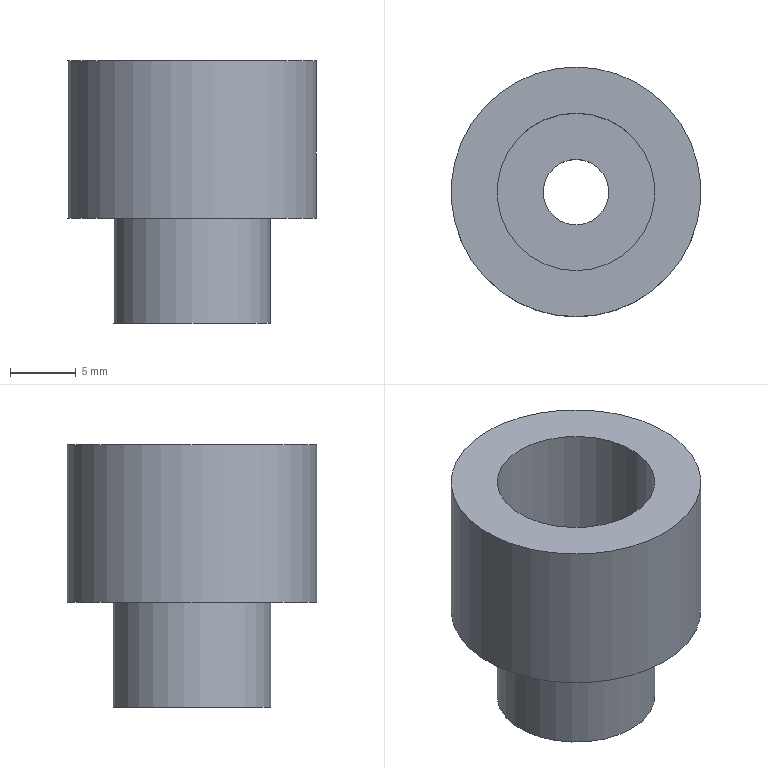Part | STEP file | 1-16.6 | 1 solid | 8 faces | box 19 x 19 x 20 mm | volume 2980 mm3 | cylinder 4 | plane 4 | commonest cylinder face diameters 12 x2 5 x1 19 x1
STEP:
#1=CARTESIAN_POINT('',(0.,0.,0.));
#2=DIRECTION('',(0.,0.,1.));
#3=DIRECTION('',(1.,0.,0.));
#4=AXIS2_PLACEMENT_3D('',#1,#2,#3);
#5=CARTESIAN_POINT('',(0.,9.5,0.));
#6=VERTEX_POINT('',#5);
#7=CARTESIAN_POINT('',(0.,0.,0.));
#8=DIRECTION('',(0.,0.,1.));
#9=DIRECTION('',(0.,1.,0.));
#10=AXIS2_PLACEMENT_3D('',#7,#8,#9);
#11=CIRCLE('',#10,9.5);
#12=CARTESIAN_POINT('',(0.,0.,0.));
#13=DIRECTION('',(0.,0.,1.));
#14=DIRECTION('',(0.,1.,0.));
#15=AXIS2_PLACEMENT_3D('',#12,#13,#14);
#16=CYLINDRICAL_SURFACE('',#15,9.5);
#17=CARTESIAN_POINT('',(0.,0.));
#18=DIRECTION('',(1.,0.));
#19=VECTOR('',#18,1.);
#20=LINE('',#17,#19);
#21=(GEOMETRIC_REPRESENTATION_CONTEXT(2)PARAMETRIC_REPRESENTATION_CONTEXT()REPRESENTATION_CONTEXT('',''));
#22=DEFINITIONAL_REPRESENTATION('',(#20),#21);
#23=PCURVE('',#16,#22);
#24=CARTESIAN_POINT('',(0.,-2.546,0.));
#25=DIRECTION('',(0.,0.,1.));
#26=DIRECTION('',(1.,0.,0.));
#27=AXIS2_PLACEMENT_3D('',#24,#25,#26);
#28=PLANE('',#27);
#29=CARTESIAN_POINT('',(0.,2.546));
#30=DIRECTION('',(0.,1.));
#31=AXIS2_PLACEMENT_2D('',#29,#30);
#32=CIRCLE('',#31,9.5);
#33=(GEOMETRIC_REPRESENTATION_CONTEXT(2)PARAMETRIC_REPRESENTATION_CONTEXT()REPRESENTATION_CONTEXT('',''));
#34=DEFINITIONAL_REPRESENTATION('',(#32),#33);
#35=PCURVE('',#28,#34);
#36=SURFACE_CURVE('',#11,(#23,#35),.PCURVE_S1.);
#37=EDGE_CURVE('',#6,#6,#36,.T.);
#38=ORIENTED_EDGE('',*,*,#37,.T.);
#39=CARTESIAN_POINT('',(0.,9.5,12.));
#40=VERTEX_POINT('',#39);
#41=CARTESIAN_POINT('',(0.,9.5,0.));
#42=DIRECTION('',(0.,0.,1.));
#43=VECTOR('',#42,1.);
#44=LINE('',#41,#43);
#45=CARTESIAN_POINT('',(6.283,0.));
#46=DIRECTION('',(0.,1.));
#47=VECTOR('',#46,1.);
#48=LINE('',#45,#47);
#49=(GEOMETRIC_REPRESENTATION_CONTEXT(2)PARAMETRIC_REPRESENTATION_CONTEXT()REPRESENTATION_CONTEXT('',''));
#50=DEFINITIONAL_REPRESENTATION('',(#48),#49);
#51=PCURVE('',#16,#50);
#52=CARTESIAN_POINT('',(0.,0.));
#53=DIRECTION('',(0.,1.));
#54=VECTOR('',#53,1.);
#55=LINE('',#52,#54);
#56=(GEOMETRIC_REPRESENTATION_CONTEXT(2)PARAMETRIC_REPRESENTATION_CONTEXT()REPRESENTATION_CONTEXT('',''));
#57=DEFINITIONAL_REPRESENTATION('',(#55),#56);
#58=PCURVE('',#16,#57);
#59=SEAM_CURVE('',#44,(#51,#58),.PCURVE_S1.);
#60=EDGE_CURVE('',#6,#40,#59,.T.);
#61=ORIENTED_EDGE('',*,*,#60,.T.);
#62=CARTESIAN_POINT('',(0.,0.,12.));
#63=DIRECTION('',(0.,0.,1.));
#64=DIRECTION('',(0.,1.,0.));
#65=AXIS2_PLACEMENT_3D('',#62,#63,#64);
#66=CIRCLE('',#65,9.5);
#67=CARTESIAN_POINT('',(0.,12.));
#68=DIRECTION('',(1.,0.));
#69=VECTOR('',#68,1.);
#70=LINE('',#67,#69);
#71=(GEOMETRIC_REPRESENTATION_CONTEXT(2)PARAMETRIC_REPRESENTATION_CONTEXT()REPRESENTATION_CONTEXT('',''));
#72=DEFINITIONAL_REPRESENTATION('',(#70),#71);
#73=PCURVE('',#16,#72);
#74=CARTESIAN_POINT('',(0.,-2.546,12.));
#75=DIRECTION('',(0.,0.,1.));
#76=DIRECTION('',(1.,0.,0.));
#77=AXIS2_PLACEMENT_3D('',#74,#75,#76);
#78=PLANE('',#77);
#79=CARTESIAN_POINT('',(0.,2.546));
#80=DIRECTION('',(0.,1.));
#81=AXIS2_PLACEMENT_2D('',#79,#80);
#82=CIRCLE('',#81,9.5);
#83=(GEOMETRIC_REPRESENTATION_CONTEXT(2)PARAMETRIC_REPRESENTATION_CONTEXT()REPRESENTATION_CONTEXT('',''));
#84=DEFINITIONAL_REPRESENTATION('',(#82),#83);
#85=PCURVE('',#78,#84);
#86=SURFACE_CURVE('',#66,(#73,#85),.PCURVE_S1.);
#87=EDGE_CURVE('',#40,#40,#86,.T.);
#88=ORIENTED_EDGE('',*,*,#87,.F.);
#89=ORIENTED_EDGE('',*,*,#60,.F.);
#90=EDGE_LOOP('',(#38,#61,#88,#89));
#91=FACE_BOUND('',#90,.T.);
#92=ADVANCED_FACE('',(#91),#16,.T.);
#93=ORIENTED_EDGE('',*,*,#37,.T.);
#94=EDGE_LOOP('',(#93));
#95=FACE_BOUND('',#94,.F.);
#96=CARTESIAN_POINT('',(0.,6.,0.));
#97=VERTEX_POINT('',#96);
#98=CARTESIAN_POINT('',(0.,0.,0.));
#99=DIRECTION('',(0.,0.,1.));
#100=DIRECTION('',(0.,1.,0.));
#101=AXIS2_PLACEMENT_3D('',#98,#99,#100);
#102=CIRCLE('',#101,6.);
#103=CARTESIAN_POINT('',(0.,2.546));
#104=DIRECTION('',(0.,1.));
#105=AXIS2_PLACEMENT_2D('',#103,#104);
#106=CIRCLE('',#105,6.);
#107=(GEOMETRIC_REPRESENTATION_CONTEXT(2)PARAMETRIC_REPRESENTATION_CONTEXT()REPRESENTATION_CONTEXT('',''));
#108=DEFINITIONAL_REPRESENTATION('',(#106),#107);
#109=PCURVE('',#28,#108);
#110=CARTESIAN_POINT('',(0.,0.,0.));
#111=DIRECTION('',(0.,0.,-1.));
#112=DIRECTION('',(0.,1.,0.));
#113=AXIS2_PLACEMENT_3D('',#110,#111,#112);
#114=CYLINDRICAL_SURFACE('',#113,6.);
#115=CARTESIAN_POINT('',(6.283,0.));
#116=DIRECTION('',(-1.,0.));
#117=VECTOR('',#116,1.);
#118=LINE('',#115,#117);
#119=(GEOMETRIC_REPRESENTATION_CONTEXT(2)PARAMETRIC_REPRESENTATION_CONTEXT()REPRESENTATION_CONTEXT('',''));
#120=DEFINITIONAL_REPRESENTATION('',(#118),#119);
#121=PCURVE('',#114,#120);
#122=SURFACE_CURVE('',#102,(#109,#121),.PCURVE_S1.);
#123=EDGE_CURVE('',#97,#97,#122,.T.);
#124=ORIENTED_EDGE('',*,*,#123,.F.);
#125=EDGE_LOOP('',(#124));
#126=FACE_BOUND('',#125,.F.);
#127=ADVANCED_FACE('',(#95,#126),#28,.F.);
#128=CARTESIAN_POINT('',(0.,6.,-8.));
#129=VERTEX_POINT('',#128);
#130=CARTESIAN_POINT('',(0.,6.,0.));
#131=DIRECTION('',(0.,0.,-1.));
#132=VECTOR('',#131,1.);
#133=LINE('',#130,#132);
#134=CARTESIAN_POINT('',(6.283,0.));
#135=DIRECTION('',(0.,1.));
#136=VECTOR('',#135,1.);
#137=LINE('',#134,#136);
#138=(GEOMETRIC_REPRESENTATION_CONTEXT(2)PARAMETRIC_REPRESENTATION_CONTEXT()REPRESENTATION_CONTEXT('',''));
#139=DEFINITIONAL_REPRESENTATION('',(#137),#138);
#140=PCURVE('',#114,#139);
#141=CARTESIAN_POINT('',(0.,0.));
#142=DIRECTION('',(0.,1.));
#143=VECTOR('',#142,1.);
#144=LINE('',#141,#143);
#145=(GEOMETRIC_REPRESENTATION_CONTEXT(2)PARAMETRIC_REPRESENTATION_CONTEXT()REPRESENTATION_CONTEXT('',''));
#146=DEFINITIONAL_REPRESENTATION('',(#144),#145);
#147=PCURVE('',#114,#146);
#148=SEAM_CURVE('',#133,(#140,#147),.PCURVE_S1.);
#149=EDGE_CURVE('',#97,#129,#148,.T.);
#150=ORIENTED_EDGE('',*,*,#149,.T.);
#151=CARTESIAN_POINT('',(0.,0.,-8.));
#152=DIRECTION('',(0.,0.,1.));
#153=DIRECTION('',(0.,1.,0.));
#154=AXIS2_PLACEMENT_3D('',#151,#152,#153);
#155=CIRCLE('',#154,6.);
#156=CARTESIAN_POINT('',(6.283,8.));
#157=DIRECTION('',(-1.,0.));
#158=VECTOR('',#157,1.);
#159=LINE('',#156,#158);
#160=(GEOMETRIC_REPRESENTATION_CONTEXT(2)PARAMETRIC_REPRESENTATION_CONTEXT()REPRESENTATION_CONTEXT('',''));
#161=DEFINITIONAL_REPRESENTATION('',(#159),#160);
#162=PCURVE('',#114,#161);
#163=CARTESIAN_POINT('',(0.,-1.608,-8.));
#164=DIRECTION('',(0.,0.,1.));
#165=DIRECTION('',(1.,0.,0.));
#166=AXIS2_PLACEMENT_3D('',#163,#164,#165);
#167=PLANE('',#166);
#168=CARTESIAN_POINT('',(0.,1.608));
#169=DIRECTION('',(0.,1.));
#170=AXIS2_PLACEMENT_2D('',#168,#169);
#171=CIRCLE('',#170,6.);
#172=(GEOMETRIC_REPRESENTATION_CONTEXT(2)PARAMETRIC_REPRESENTATION_CONTEXT()REPRESENTATION_CONTEXT('',''));
#173=DEFINITIONAL_REPRESENTATION('',(#171),#172);
#174=PCURVE('',#167,#173);
#175=SURFACE_CURVE('',#155,(#162,#174),.PCURVE_S1.);
#176=EDGE_CURVE('',#129,#129,#175,.T.);
#177=ORIENTED_EDGE('',*,*,#176,.T.);
#178=ORIENTED_EDGE('',*,*,#149,.F.);
#179=ORIENTED_EDGE('',*,*,#123,.F.);
#180=EDGE_LOOP('',(#150,#177,#178,#179));
#181=FACE_BOUND('',#180,.T.);
#182=ADVANCED_FACE('',(#181),#114,.T.);
#183=ORIENTED_EDGE('',*,*,#87,.T.);
#184=EDGE_LOOP('',(#183));
#185=FACE_BOUND('',#184,.T.);
#186=CARTESIAN_POINT('',(0.,6.,12.));
#187=VERTEX_POINT('',#186);
#188=CARTESIAN_POINT('',(0.,0.,12.));
#189=DIRECTION('',(0.,0.,1.));
#190=DIRECTION('',(0.,1.,0.));
#191=AXIS2_PLACEMENT_3D('',#188,#189,#190);
#192=CIRCLE('',#191,6.);
#193=CARTESIAN_POINT('',(0.,2.546));
#194=DIRECTION('',(0.,1.));
#195=AXIS2_PLACEMENT_2D('',#193,#194);
#196=CIRCLE('',#195,6.);
#197=(GEOMETRIC_REPRESENTATION_CONTEXT(2)PARAMETRIC_REPRESENTATION_CONTEXT()REPRESENTATION_CONTEXT('',''));
#198=DEFINITIONAL_REPRESENTATION('',(#196),#197);
#199=PCURVE('',#78,#198);
#200=CARTESIAN_POINT('',(0.,0.,12.));
#201=DIRECTION('',(0.,0.,-1.));
#202=DIRECTION('',(0.,1.,0.));
#203=AXIS2_PLACEMENT_3D('',#200,#201,#202);
#204=CYLINDRICAL_SURFACE('',#203,6.);
#205=CARTESIAN_POINT('',(6.283,0.));
#206=DIRECTION('',(-1.,0.));
#207=VECTOR('',#206,1.);
#208=LINE('',#205,#207);
#209=(GEOMETRIC_REPRESENTATION_CONTEXT(2)PARAMETRIC_REPRESENTATION_CONTEXT()REPRESENTATION_CONTEXT('',''));
#210=DEFINITIONAL_REPRESENTATION('',(#208),#209);
#211=PCURVE('',#204,#210);
#212=SURFACE_CURVE('',#192,(#199,#211),.PCURVE_S1.);
#213=EDGE_CURVE('',#187,#187,#212,.T.);
#214=ORIENTED_EDGE('',*,*,#213,.F.);
#215=EDGE_LOOP('',(#214));
#216=FACE_BOUND('',#215,.T.);
#217=ADVANCED_FACE('',(#185,#216),#78,.T.);
#218=CARTESIAN_POINT('',(0.,6.,2.));
#219=VERTEX_POINT('',#218);
#220=CARTESIAN_POINT('',(0.,6.,12.));
#221=DIRECTION('',(0.,0.,-1.));
#222=VECTOR('',#221,1.);
#223=LINE('',#220,#222);
#224=CARTESIAN_POINT('',(6.283,0.));
#225=DIRECTION('',(0.,1.));
#226=VECTOR('',#225,1.);
#227=LINE('',#224,#226);
#228=(GEOMETRIC_REPRESENTATION_CONTEXT(2)PARAMETRIC_REPRESENTATION_CONTEXT()REPRESENTATION_CONTEXT('',''));
#229=DEFINITIONAL_REPRESENTATION('',(#227),#228);
#230=PCURVE('',#204,#229);
#231=CARTESIAN_POINT('',(0.,0.));
#232=DIRECTION('',(0.,1.));
#233=VECTOR('',#232,1.);
#234=LINE('',#231,#233);
#235=(GEOMETRIC_REPRESENTATION_CONTEXT(2)PARAMETRIC_REPRESENTATION_CONTEXT()REPRESENTATION_CONTEXT('',''));
#236=DEFINITIONAL_REPRESENTATION('',(#234),#235);
#237=PCURVE('',#204,#236);
#238=SEAM_CURVE('',#223,(#230,#237),.PCURVE_S1.);
#239=EDGE_CURVE('',#187,#219,#238,.T.);
#240=ORIENTED_EDGE('',*,*,#239,.T.);
#241=CARTESIAN_POINT('',(0.,0.,2.));
#242=DIRECTION('',(0.,0.,1.));
#243=DIRECTION('',(0.,1.,0.));
#244=AXIS2_PLACEMENT_3D('',#241,#242,#243);
#245=CIRCLE('',#244,6.);
#246=CARTESIAN_POINT('',(6.283,10.));
#247=DIRECTION('',(-1.,0.));
#248=VECTOR('',#247,1.);
#249=LINE('',#246,#248);
#250=(GEOMETRIC_REPRESENTATION_CONTEXT(2)PARAMETRIC_REPRESENTATION_CONTEXT()REPRESENTATION_CONTEXT('',''));
#251=DEFINITIONAL_REPRESENTATION('',(#249),#250);
#252=PCURVE('',#204,#251);
#253=CARTESIAN_POINT('',(0.,-1.608,2.));
#254=DIRECTION('',(0.,0.,1.));
#255=DIRECTION('',(1.,0.,0.));
#256=AXIS2_PLACEMENT_3D('',#253,#254,#255);
#257=PLANE('',#256);
#258=CARTESIAN_POINT('',(0.,1.608));
#259=DIRECTION('',(0.,1.));
#260=AXIS2_PLACEMENT_2D('',#258,#259);
#261=CIRCLE('',#260,6.);
#262=(GEOMETRIC_REPRESENTATION_CONTEXT(2)PARAMETRIC_REPRESENTATION_CONTEXT()REPRESENTATION_CONTEXT('',''));
#263=DEFINITIONAL_REPRESENTATION('',(#261),#262);
#264=PCURVE('',#257,#263);
#265=SURFACE_CURVE('',#245,(#252,#264),.PCURVE_S1.);
#266=EDGE_CURVE('',#219,#219,#265,.T.);
#267=ORIENTED_EDGE('',*,*,#266,.T.);
#268=ORIENTED_EDGE('',*,*,#239,.F.);
#269=ORIENTED_EDGE('',*,*,#213,.F.);
#270=EDGE_LOOP('',(#240,#267,#268,#269));
#271=FACE_BOUND('',#270,.F.);
#272=ADVANCED_FACE('',(#271),#204,.F.);
#273=ORIENTED_EDGE('',*,*,#176,.T.);
#274=EDGE_LOOP('',(#273));
#275=FACE_BOUND('',#274,.F.);
#276=CARTESIAN_POINT('',(0.,2.5,-8.));
#277=VERTEX_POINT('',#276);
#278=CARTESIAN_POINT('',(0.,0.,-8.));
#279=DIRECTION('',(0.,0.,1.));
#280=DIRECTION('',(0.,1.,0.));
#281=AXIS2_PLACEMENT_3D('',#278,#279,#280);
#282=CIRCLE('',#281,2.5);
#283=CARTESIAN_POINT('',(0.,1.608));
#284=DIRECTION('',(0.,1.));
#285=AXIS2_PLACEMENT_2D('',#283,#284);
#286=CIRCLE('',#285,2.5);
#287=(GEOMETRIC_REPRESENTATION_CONTEXT(2)PARAMETRIC_REPRESENTATION_CONTEXT()REPRESENTATION_CONTEXT('',''));
#288=DEFINITIONAL_REPRESENTATION('',(#286),#287);
#289=PCURVE('',#167,#288);
#290=CARTESIAN_POINT('',(0.,0.,12.));
#291=DIRECTION('',(0.,0.,-1.));
#292=DIRECTION('',(0.,1.,0.));
#293=AXIS2_PLACEMENT_3D('',#290,#291,#292);
#294=CYLINDRICAL_SURFACE('',#293,2.5);
#295=CARTESIAN_POINT('',(6.283,20.));
#296=DIRECTION('',(-1.,0.));
#297=VECTOR('',#296,1.);
#298=LINE('',#295,#297);
#299=(GEOMETRIC_REPRESENTATION_CONTEXT(2)PARAMETRIC_REPRESENTATION_CONTEXT()REPRESENTATION_CONTEXT('',''));
#300=DEFINITIONAL_REPRESENTATION('',(#298),#299);
#301=PCURVE('',#294,#300);
#302=SURFACE_CURVE('',#282,(#289,#301),.PCURVE_S1.);
#303=EDGE_CURVE('',#277,#277,#302,.T.);
#304=ORIENTED_EDGE('',*,*,#303,.F.);
#305=EDGE_LOOP('',(#304));
#306=FACE_BOUND('',#305,.F.);
#307=ADVANCED_FACE('',(#275,#306),#167,.F.);
#308=ORIENTED_EDGE('',*,*,#266,.T.);
#309=EDGE_LOOP('',(#308));
#310=FACE_BOUND('',#309,.T.);
#311=CARTESIAN_POINT('',(0.,2.5,2.));
#312=VERTEX_POINT('',#311);
#313=CARTESIAN_POINT('',(0.,0.,2.));
#314=DIRECTION('',(0.,0.,1.));
#315=DIRECTION('',(0.,1.,0.));
#316=AXIS2_PLACEMENT_3D('',#313,#314,#315);
#317=CIRCLE('',#316,2.5);
#318=CARTESIAN_POINT('',(0.,1.608));
#319=DIRECTION('',(0.,1.));
#320=AXIS2_PLACEMENT_2D('',#318,#319);
#321=CIRCLE('',#320,2.5);
#322=(GEOMETRIC_REPRESENTATION_CONTEXT(2)PARAMETRIC_REPRESENTATION_CONTEXT()REPRESENTATION_CONTEXT('',''));
#323=DEFINITIONAL_REPRESENTATION('',(#321),#322);
#324=PCURVE('',#257,#323);
#325=CARTESIAN_POINT('',(6.283,10.));
#326=DIRECTION('',(-1.,0.));
#327=VECTOR('',#326,1.);
#328=LINE('',#325,#327);
#329=(GEOMETRIC_REPRESENTATION_CONTEXT(2)PARAMETRIC_REPRESENTATION_CONTEXT()REPRESENTATION_CONTEXT('',''));
#330=DEFINITIONAL_REPRESENTATION('',(#328),#329);
#331=PCURVE('',#294,#330);
#332=SURFACE_CURVE('',#317,(#324,#331),.PCURVE_S1.);
#333=EDGE_CURVE('',#312,#312,#332,.T.);
#334=ORIENTED_EDGE('',*,*,#333,.F.);
#335=EDGE_LOOP('',(#334));
#336=FACE_BOUND('',#335,.T.);
#337=ADVANCED_FACE('',(#310,#336),#257,.T.);
#338=CARTESIAN_POINT('',(0.,2.5,2.));
#339=DIRECTION('',(0.,0.,-1.));
#340=VECTOR('',#339,1.);
#341=LINE('',#338,#340);
#342=CARTESIAN_POINT('',(0.,10.));
#343=DIRECTION('',(0.,1.));
#344=VECTOR('',#343,1.);
#345=LINE('',#342,#344);
#346=(GEOMETRIC_REPRESENTATION_CONTEXT(2)PARAMETRIC_REPRESENTATION_CONTEXT()REPRESENTATION_CONTEXT('',''));
#347=DEFINITIONAL_REPRESENTATION('',(#345),#346);
#348=PCURVE('',#294,#347);
#349=CARTESIAN_POINT('',(6.283,10.));
#350=DIRECTION('',(0.,1.));
#351=VECTOR('',#350,1.);
#352=LINE('',#349,#351);
#353=(GEOMETRIC_REPRESENTATION_CONTEXT(2)PARAMETRIC_REPRESENTATION_CONTEXT()REPRESENTATION_CONTEXT('',''));
#354=DEFINITIONAL_REPRESENTATION('',(#352),#353);
#355=PCURVE('',#294,#354);
#356=SEAM_CURVE('',#341,(#348,#355),.PCURVE_S1.);
#357=EDGE_CURVE('',#312,#277,#356,.T.);
#358=ORIENTED_EDGE('',*,*,#357,.F.);
#359=ORIENTED_EDGE('',*,*,#333,.F.);
#360=ORIENTED_EDGE('',*,*,#357,.T.);
#361=ORIENTED_EDGE('',*,*,#303,.T.);
#362=EDGE_LOOP('',(#358,#359,#360,#361));
#363=FACE_BOUND('',#362,.F.);
#364=ADVANCED_FACE('',(#363),#294,.F.);
#365=CLOSED_SHELL('',(#92,#127,#182,#217,#272,#307,#337,#364));
#366=MANIFOLD_SOLID_BREP('',#365);
#367=(LENGTH_UNIT()NAMED_UNIT(*)SI_UNIT(.MILLI.,.METRE.));
#368=UNCERTAINTY_MEASURE_WITH_UNIT(LENGTH_MEASURE(0.0000001),#367,'','');
#369=(NAMED_UNIT(*)PLANE_ANGLE_UNIT()SI_UNIT($,.RADIAN.));
#370=(NAMED_UNIT(*)SI_UNIT($,.STERADIAN.)SOLID_ANGLE_UNIT());
#371=(GEOMETRIC_REPRESENTATION_CONTEXT(3)GLOBAL_UNCERTAINTY_ASSIGNED_CONTEXT((#368))GLOBAL_UNIT_ASSIGNED_CONTEXT((#367,#369,#370))REPRESENTATION_CONTEXT('',''));
#372=ADVANCED_BREP_SHAPE_REPRESENTATION('',(#4,#366),#371);